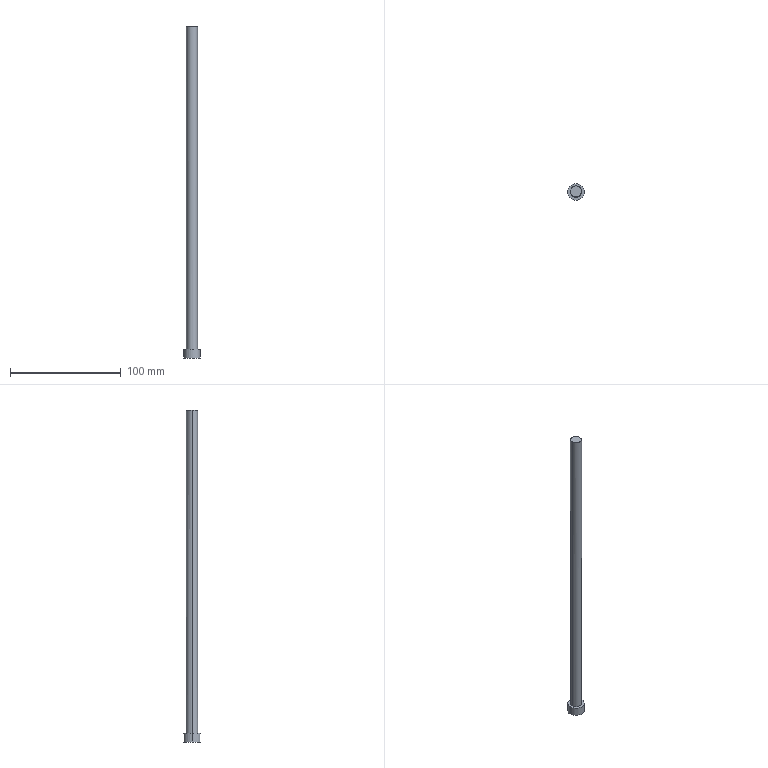Part | Creo | 1 solid | 10 faces | box 15 x 15 x 299.18 mm | volume 24214 mm3 | cylinder 6 | plane 4 | commonest cylinder face diameters 3 x2 10 x2 15 x2
STEP:
#1=CARTESIAN_POINT('',(-84.,203.,38.298));
#2=VERTEX_POINT('',#1);
#3=CARTESIAN_POINT('',(-94.,203.,38.68));
#4=VERTEX_POINT('',#3);
#5=CARTESIAN_POINT('',(-84.,203.,38.298));
#6=CARTESIAN_POINT('',(-84.,202.411,38.298));
#7=CARTESIAN_POINT('',(-84.215,201.138,38.306));
#8=CARTESIAN_POINT('',(-85.355,199.359,38.35));
#9=CARTESIAN_POINT('',(-87.15,198.214,38.418));
#10=CARTESIAN_POINT('',(-89.,197.893,38.489));
#11=CARTESIAN_POINT('',(-90.85,198.214,38.559));
#12=CARTESIAN_POINT('',(-92.645,199.359,38.628));
#13=CARTESIAN_POINT('',(-93.785,201.138,38.672));
#14=CARTESIAN_POINT('',(-94.,202.411,38.68));
#15=CARTESIAN_POINT('',(-94.,203.,38.68));
#16=B_SPLINE_CURVE_WITH_KNOTS('',3,(#5,#6,#7,#8,#9,#10,#11,#12,#13,#14,#15),.UNSPECIFIED.,.F.,.F.,(4,1,1,1,1,1,1,1,4),(0.,0.125,0.25,0.375,0.5,0.625,0.75,0.875,1.),.UNSPECIFIED.);
#17=EDGE_CURVE('',#2,#4,#16,.T.);
#18=ORIENTED_EDGE('',*,*,#17,.F.);
#19=CARTESIAN_POINT('',(-84.,203.,-252.5));
#20=VERTEX_POINT('',#19);
#21=CARTESIAN_POINT('',(-84.,203.,38.298));
#22=DIRECTION('',(0.,0.,-1.));
#23=VECTOR('',#22,290.798);
#24=LINE('',#21,#23);
#25=EDGE_CURVE('',#2,#20,#24,.T.);
#26=ORIENTED_EDGE('',*,*,#25,.T.);
#27=CARTESIAN_POINT('',(-94.,203.,-252.5));
#28=VERTEX_POINT('',#27);
#29=CARTESIAN_POINT('',(-89.,203.,-252.5));
#30=DIRECTION('',(0.,0.,-1.));
#31=DIRECTION('',(1.,0.,0.));
#32=AXIS2_PLACEMENT_3D('',#29,#30,#31);
#33=CIRCLE('',#32,5.);
#34=EDGE_CURVE('',#20,#28,#33,.T.);
#35=ORIENTED_EDGE('',*,*,#34,.T.);
#36=CARTESIAN_POINT('',(-94.,203.,38.68));
#37=DIRECTION('',(0.,0.,-1.));
#38=VECTOR('',#37,291.18);
#39=LINE('',#36,#38);
#40=EDGE_CURVE('',#4,#28,#39,.T.);
#41=ORIENTED_EDGE('',*,*,#40,.F.);
#42=EDGE_LOOP('',(#18,#26,#35,#41));
#43=FACE_OUTER_BOUND('',#42,.F.);
#44=CARTESIAN_POINT('',(-89.,203.,135.));
#45=DIRECTION('',(0.,0.,-1.));
#46=DIRECTION('',(1.,0.,0.));
#47=AXIS2_PLACEMENT_3D('',#44,#45,#46);
#48=CYLINDRICAL_SURFACE('',#47,5.);
#49=ADVANCED_FACE('',(#43),#48,.T.);
#50=CARTESIAN_POINT('',(-94.,203.,38.68));
#51=CARTESIAN_POINT('',(-94.,203.589,38.68));
#52=CARTESIAN_POINT('',(-93.785,204.862,38.672));
#53=CARTESIAN_POINT('',(-92.645,206.641,38.628));
#54=CARTESIAN_POINT('',(-90.85,207.786,38.559));
#55=CARTESIAN_POINT('',(-89.,208.107,38.489));
#56=CARTESIAN_POINT('',(-87.15,207.786,38.418));
#57=CARTESIAN_POINT('',(-85.355,206.641,38.35));
#58=CARTESIAN_POINT('',(-84.215,204.862,38.306));
#59=CARTESIAN_POINT('',(-84.,203.589,38.298));
#60=CARTESIAN_POINT('',(-84.,203.,38.298));
#61=B_SPLINE_CURVE_WITH_KNOTS('',3,(#50,#51,#52,#53,#54,#55,#56,#57,#58,#59,#60),.UNSPECIFIED.,.F.,.F.,(4,1,1,1,1,1,1,1,4),(0.,0.125,0.25,0.375,0.5,0.625,0.75,0.875,1.),.UNSPECIFIED.);
#62=EDGE_CURVE('',#4,#2,#61,.T.);
#63=ORIENTED_EDGE('',*,*,#62,.T.);
#64=ORIENTED_EDGE('',*,*,#17,.T.);
#65=EDGE_LOOP('',(#63,#64));
#66=FACE_OUTER_BOUND('',#65,.F.);
#67=CARTESIAN_POINT('',(-122.791,-167.242,39.779));
#68=DIRECTION('',(-0.03814,0.,-0.9993));
#69=DIRECTION('',(-0.9993,0.,0.03814));
#70=AXIS2_PLACEMENT_3D('',#67,#68,#69);
#71=PLANE('',#70);
#72=ADVANCED_FACE('',(#66),#71,.F.);
#73=ORIENTED_EDGE('',*,*,#62,.F.);
#74=ORIENTED_EDGE('',*,*,#40,.T.);
#75=CARTESIAN_POINT('',(-89.,203.,-252.5));
#76=DIRECTION('',(0.,0.,-1.));
#77=DIRECTION('',(-1.,0.,0.));
#78=AXIS2_PLACEMENT_3D('',#75,#76,#77);
#79=CIRCLE('',#78,5.);
#80=EDGE_CURVE('',#28,#20,#79,.T.);
#81=ORIENTED_EDGE('',*,*,#80,.T.);
#82=ORIENTED_EDGE('',*,*,#25,.F.);
#83=EDGE_LOOP('',(#73,#74,#81,#82));
#84=FACE_OUTER_BOUND('',#83,.F.);
#85=CARTESIAN_POINT('',(-89.,203.,135.));
#86=DIRECTION('',(0.,0.,-1.));
#87=DIRECTION('',(1.,0.,0.));
#88=AXIS2_PLACEMENT_3D('',#85,#86,#87);
#89=CYLINDRICAL_SURFACE('',#88,5.);
#90=ADVANCED_FACE('',(#84),#89,.T.);
#91=CARTESIAN_POINT('',(-96.5,203.,-252.5));
#92=VERTEX_POINT('',#91);
#93=CARTESIAN_POINT('',(-81.5,203.,-252.5));
#94=VERTEX_POINT('',#93);
#95=CARTESIAN_POINT('',(-89.,203.,-252.5));
#96=DIRECTION('',(0.,0.,1.));
#97=DIRECTION('',(-1.,0.,0.));
#98=AXIS2_PLACEMENT_3D('',#95,#96,#97);
#99=CIRCLE('',#98,7.5);
#100=EDGE_CURVE('',#92,#94,#99,.T.);
#101=ORIENTED_EDGE('',*,*,#100,.F.);
#102=CARTESIAN_POINT('',(-89.,203.,-252.5));
#103=DIRECTION('',(0.,0.,1.));
#104=DIRECTION('',(1.,0.,0.));
#105=AXIS2_PLACEMENT_3D('',#102,#103,#104);
#106=CIRCLE('',#105,7.5);
#107=EDGE_CURVE('',#94,#92,#106,.T.);
#108=ORIENTED_EDGE('',*,*,#107,.F.);
#109=EDGE_LOOP('',(#101,#108));
#110=FACE_OUTER_BOUND('',#109,.F.);
#111=ORIENTED_EDGE('',*,*,#80,.F.);
#112=ORIENTED_EDGE('',*,*,#34,.F.);
#113=EDGE_LOOP('',(#111,#112));
#114=FACE_BOUND('',#113,.F.);
#115=CARTESIAN_POINT('',(-89.,203.,-252.5));
#116=DIRECTION('',(0.,0.,1.));
#117=DIRECTION('',(-1.,0.,0.));
#118=AXIS2_PLACEMENT_3D('',#115,#116,#117);
#119=PLANE('',#118);
#120=ADVANCED_FACE('',(#110,#114),#119,.T.);
#121=CARTESIAN_POINT('',(-81.5,203.,-258.));
#122=VERTEX_POINT('',#121);
#123=CARTESIAN_POINT('',(-81.5,203.,-255.));
#124=VERTEX_POINT('',#123);
#125=CARTESIAN_POINT('',(-81.5,203.,-258.));
#126=CARTESIAN_POINT('',(-81.5,202.795,-258.));
#127=CARTESIAN_POINT('',(-81.516,202.417,-257.922));
#128=CARTESIAN_POINT('',(-81.575,201.91,-257.589));
#129=CARTESIAN_POINT('',(-81.635,201.576,-257.085));
#130=CARTESIAN_POINT('',(-81.66,201.461,-256.497));
#131=CARTESIAN_POINT('',(-81.635,201.578,-255.912));
#132=CARTESIAN_POINT('',(-81.575,201.909,-255.413));
#133=CARTESIAN_POINT('',(-81.516,202.415,-255.078));
#134=CARTESIAN_POINT('',(-81.5,202.794,-255.));
#135=CARTESIAN_POINT('',(-81.5,203.,-255.));
#136=B_SPLINE_CURVE_WITH_KNOTS('',3,(#125,#126,#127,#128,#129,#130,#131,#132,#133,#134,#135),.UNSPECIFIED.,.F.,.F.,(4,1,1,1,1,1,1,1,4),(0.,0.125,0.25,0.375,0.5,0.625,0.75,0.875,1.),.UNSPECIFIED.);
#137=EDGE_CURVE('',#122,#124,#136,.T.);
#138=ORIENTED_EDGE('',*,*,#137,.F.);
#139=CARTESIAN_POINT('',(-81.5,203.,-260.5));
#140=VERTEX_POINT('',#139);
#141=CARTESIAN_POINT('',(-81.5,203.,-260.5));
#142=DIRECTION('',(0.,0.,1.));
#143=VECTOR('',#142,2.5);
#144=LINE('',#141,#143);
#145=EDGE_CURVE('',#140,#122,#144,.T.);
#146=ORIENTED_EDGE('',*,*,#145,.F.);
#147=CARTESIAN_POINT('',(-96.5,203.,-260.5));
#148=VERTEX_POINT('',#147);
#149=CARTESIAN_POINT('',(-89.,203.,-260.5));
#150=DIRECTION('',(0.,0.,-1.));
#151=DIRECTION('',(1.,0.,0.));
#152=AXIS2_PLACEMENT_3D('',#149,#150,#151);
#153=CIRCLE('',#152,7.5);
#154=EDGE_CURVE('',#140,#148,#153,.T.);
#155=ORIENTED_EDGE('',*,*,#154,.T.);
#156=CARTESIAN_POINT('',(-96.5,203.,-260.5));
#157=DIRECTION('',(0.,0.,1.));
#158=VECTOR('',#157,8.);
#159=LINE('',#156,#158);
#160=EDGE_CURVE('',#148,#92,#159,.T.);
#161=ORIENTED_EDGE('',*,*,#160,.T.);
#162=ORIENTED_EDGE('',*,*,#100,.T.);
#163=CARTESIAN_POINT('',(-81.5,203.,-255.));
#164=DIRECTION('',(0.000005138,0.,1.));
#165=VECTOR('',#164,2.5);
#166=LINE('',#163,#165);
#167=EDGE_CURVE('',#124,#94,#166,.T.);
#168=ORIENTED_EDGE('',*,*,#167,.F.);
#169=EDGE_LOOP('',(#138,#146,#155,#161,#162,#168));
#170=FACE_OUTER_BOUND('',#169,.F.);
#171=CARTESIAN_POINT('',(-89.,203.,-260.5));
#172=DIRECTION('',(0.,0.,1.));
#173=DIRECTION('',(-1.,0.,0.));
#174=AXIS2_PLACEMENT_3D('',#171,#172,#173);
#175=CYLINDRICAL_SURFACE('',#174,7.5);
#176=ADVANCED_FACE('',(#170),#175,.T.);
#177=ORIENTED_EDGE('',*,*,#137,.T.);
#178=CARTESIAN_POINT('',(-89.,203.,-255.));
#179=VERTEX_POINT('',#178);
#180=CARTESIAN_POINT('',(-89.,203.,-255.));
#181=DIRECTION('',(1.,0.,-0.000004561));
#182=VECTOR('',#181,7.5);
#183=LINE('',#180,#182);
#184=EDGE_CURVE('',#179,#124,#183,.T.);
#185=ORIENTED_EDGE('',*,*,#184,.F.);
#186=CARTESIAN_POINT('',(-89.,203.,-258.));
#187=VERTEX_POINT('',#186);
#188=CARTESIAN_POINT('',(-89.,203.,-256.5));
#189=DIRECTION('',(1.,0.,0.));
#190=DIRECTION('',(0.,0.,1.));
#191=AXIS2_PLACEMENT_3D('',#188,#189,#190);
#192=CIRCLE('',#191,1.5);
#193=EDGE_CURVE('',#179,#187,#192,.T.);
#194=ORIENTED_EDGE('',*,*,#193,.T.);
#195=CARTESIAN_POINT('',(-89.,203.,-258.));
#196=DIRECTION('',(1.,0.,0.));
#197=VECTOR('',#196,7.5);
#198=LINE('',#195,#197);
#199=EDGE_CURVE('',#187,#122,#198,.T.);
#200=ORIENTED_EDGE('',*,*,#199,.T.);
#201=EDGE_LOOP('',(#177,#185,#194,#200));
#202=FACE_OUTER_BOUND('',#201,.F.);
#203=CARTESIAN_POINT('',(-89.,203.,-256.5));
#204=DIRECTION('',(1.,0.,0.));
#205=DIRECTION('',(0.,0.,-1.));
#206=AXIS2_PLACEMENT_3D('',#203,#204,#205);
#207=CYLINDRICAL_SURFACE('',#206,1.5);
#208=ADVANCED_FACE('',(#202),#207,.F.);
#209=CARTESIAN_POINT('',(-81.5,203.,-255.));
#210=CARTESIAN_POINT('',(-81.5,203.206,-255.));
#211=CARTESIAN_POINT('',(-81.516,203.585,-255.078));
#212=CARTESIAN_POINT('',(-81.576,204.093,-255.414));
#213=CARTESIAN_POINT('',(-81.636,204.424,-255.917));
#214=CARTESIAN_POINT('',(-81.66,204.539,-256.506));
#215=CARTESIAN_POINT('',(-81.635,204.421,-257.089));
#216=CARTESIAN_POINT('',(-81.576,204.092,-257.586));
#217=CARTESIAN_POINT('',(-81.516,203.586,-257.922));
#218=CARTESIAN_POINT('',(-81.5,203.206,-258.));
#219=CARTESIAN_POINT('',(-81.5,203.,-258.));
#220=B_SPLINE_CURVE_WITH_KNOTS('',3,(#209,#210,#211,#212,#213,#214,#215,#216,#217,#218,#219),.UNSPECIFIED.,.F.,.F.,(4,1,1,1,1,1,1,1,4),(0.,0.125,0.25,0.375,0.5,0.625,0.75,0.875,1.),.UNSPECIFIED.);
#221=EDGE_CURVE('',#124,#122,#220,.T.);
#222=ORIENTED_EDGE('',*,*,#221,.T.);
#223=ORIENTED_EDGE('',*,*,#199,.F.);
#224=CARTESIAN_POINT('',(-89.,203.,-256.5));
#225=DIRECTION('',(1.,0.,0.));
#226=DIRECTION('',(0.,0.,-1.));
#227=AXIS2_PLACEMENT_3D('',#224,#225,#226);
#228=CIRCLE('',#227,1.5);
#229=EDGE_CURVE('',#187,#179,#228,.T.);
#230=ORIENTED_EDGE('',*,*,#229,.T.);
#231=ORIENTED_EDGE('',*,*,#184,.T.);
#232=EDGE_LOOP('',(#222,#223,#230,#231));
#233=FACE_OUTER_BOUND('',#232,.F.);
#234=CARTESIAN_POINT('',(-89.,203.,-256.5));
#235=DIRECTION('',(1.,0.,0.));
#236=DIRECTION('',(0.,0.,-1.));
#237=AXIS2_PLACEMENT_3D('',#234,#235,#236);
#238=CYLINDRICAL_SURFACE('',#237,1.5);
#239=ADVANCED_FACE('',(#233),#238,.F.);
#240=ORIENTED_EDGE('',*,*,#221,.F.);
#241=ORIENTED_EDGE('',*,*,#167,.T.);
#242=ORIENTED_EDGE('',*,*,#107,.T.);
#243=ORIENTED_EDGE('',*,*,#160,.F.);
#244=CARTESIAN_POINT('',(-89.,203.,-260.5));
#245=DIRECTION('',(0.,0.,-1.));
#246=DIRECTION('',(-1.,0.,0.));
#247=AXIS2_PLACEMENT_3D('',#244,#245,#246);
#248=CIRCLE('',#247,7.5);
#249=EDGE_CURVE('',#148,#140,#248,.T.);
#250=ORIENTED_EDGE('',*,*,#249,.T.);
#251=ORIENTED_EDGE('',*,*,#145,.T.);
#252=EDGE_LOOP('',(#240,#241,#242,#243,#250,#251));
#253=FACE_OUTER_BOUND('',#252,.F.);
#254=CARTESIAN_POINT('',(-89.,203.,-260.5));
#255=DIRECTION('',(0.,0.,1.));
#256=DIRECTION('',(-1.,0.,0.));
#257=AXIS2_PLACEMENT_3D('',#254,#255,#256);
#258=CYLINDRICAL_SURFACE('',#257,7.5);
#259=ADVANCED_FACE('',(#253),#258,.T.);
#260=ORIENTED_EDGE('',*,*,#154,.F.);
#261=ORIENTED_EDGE('',*,*,#249,.F.);
#262=EDGE_LOOP('',(#260,#261));
#263=FACE_OUTER_BOUND('',#262,.F.);
#264=CARTESIAN_POINT('',(173.714,345.015,-260.5));
#265=DIRECTION('',(0.,0.,-1.));
#266=DIRECTION('',(1.,0.,0.));
#267=AXIS2_PLACEMENT_3D('',#264,#265,#266);
#268=PLANE('',#267);
#269=ADVANCED_FACE('',(#263),#268,.T.);
#270=ORIENTED_EDGE('',*,*,#229,.F.);
#271=ORIENTED_EDGE('',*,*,#193,.F.);
#272=EDGE_LOOP('',(#270,#271));
#273=FACE_OUTER_BOUND('',#272,.F.);
#274=CARTESIAN_POINT('',(-89.,203.,-256.5));
#275=DIRECTION('',(-1.,0.,0.));
#276=DIRECTION('',(0.,0.,1.));
#277=AXIS2_PLACEMENT_3D('',#274,#275,#276);
#278=PLANE('',#277);
#279=ADVANCED_FACE('',(#273),#278,.F.);
#280=CLOSED_SHELL('',(#49,#72,#90,#120,#176,#208,#239,#259,#269,#279));
#281=MANIFOLD_SOLID_BREP('',#280);
#282=(LENGTH_UNIT()NAMED_UNIT(*)SI_UNIT(.MILLI.,.METRE.));
#283=UNCERTAINTY_MEASURE_WITH_UNIT(LENGTH_MEASURE(0.02999),#282,'','');
#284=(NAMED_UNIT(*)PLANE_ANGLE_UNIT()SI_UNIT($,.RADIAN.));
#285=PLANE_ANGLE_MEASURE_WITH_UNIT(PLANE_ANGLE_MEASURE(0.01745),#284);
#286=(CONVERSION_BASED_UNIT('DEGREE',#285)NAMED_UNIT(*)PLANE_ANGLE_UNIT());
#287=(NAMED_UNIT(*)SI_UNIT($,.STERADIAN.)SOLID_ANGLE_UNIT());
#288=(GEOMETRIC_REPRESENTATION_CONTEXT(3)GLOBAL_UNCERTAINTY_ASSIGNED_CONTEXT((#283))GLOBAL_UNIT_ASSIGNED_CONTEXT((#282,#286,#287))REPRESENTATION_CONTEXT('',''));
#289=ADVANCED_BREP_SHAPE_REPRESENTATION('',(#281),#288);